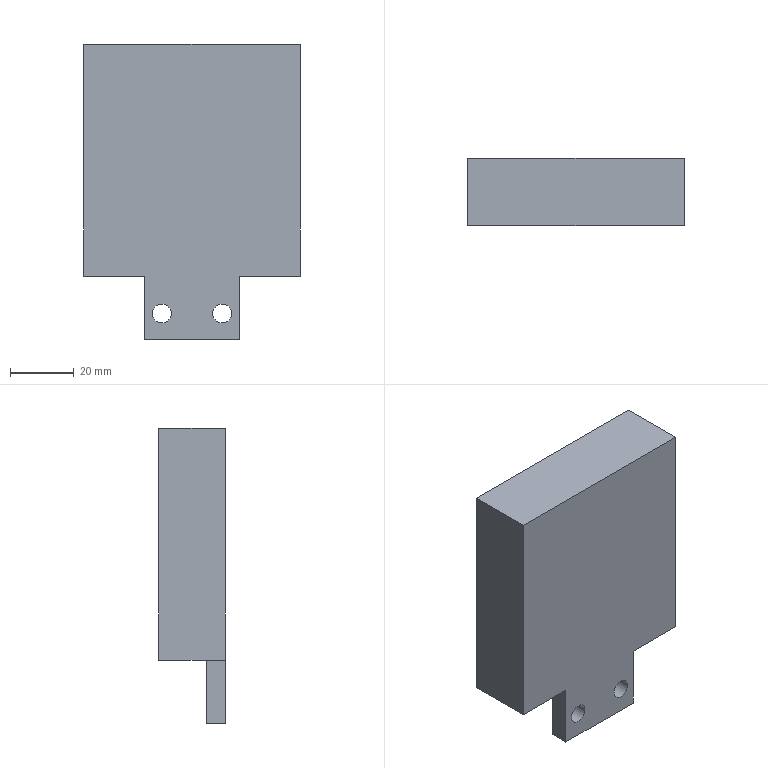Part | SolidWorks | features ICE 2, Extrusion 1 | 1 solid | 14 faces | box 68 x 21 x 93 mm | volume 107516 mm3 | plane 10 | cylinder 4 | commonest cylinder face diameters 6 x4
STEP:
#1=CARTESIAN_POINT('',(6.5,0.,-48.257));
#2=VERTEX_POINT('',#1);
#3=CARTESIAN_POINT('',(12.5,0.,-48.257));
#4=VERTEX_POINT('',#3);
#5=CARTESIAN_POINT('',(9.5,0.,-48.257));
#6=DIRECTION('',(0.,-1.,0.));
#7=DIRECTION('',(0.,0.,-1.));
#8=AXIS2_PLACEMENT_3D('',#5,#6,#7);
#9=CIRCLE('',#8,3.);
#10=EDGE_CURVE('',#2,#4,#9,.T.);
#11=ORIENTED_EDGE('',*,*,#10,.T.);
#12=CARTESIAN_POINT('',(12.5,6.02,-48.257));
#13=VERTEX_POINT('',#12);
#14=CARTESIAN_POINT('',(12.5,-13.98,-48.257));
#15=DIRECTION('',(0.,1.,0.));
#16=VECTOR('',#15,1000.);
#17=LINE('',#14,#16);
#18=EDGE_CURVE('',#4,#13,#17,.T.);
#19=ORIENTED_EDGE('',*,*,#18,.T.);
#20=CARTESIAN_POINT('',(6.5,6.02,-48.257));
#21=VERTEX_POINT('',#20);
#22=CARTESIAN_POINT('',(9.5,6.02,-48.257));
#23=DIRECTION('',(0.,1.,0.));
#24=DIRECTION('',(-1.,0.,0.));
#25=AXIS2_PLACEMENT_3D('',#22,#23,#24);
#26=CIRCLE('',#25,3.);
#27=EDGE_CURVE('',#13,#21,#26,.T.);
#28=ORIENTED_EDGE('',*,*,#27,.T.);
#29=CARTESIAN_POINT('',(6.5,-13.98,-48.257));
#30=DIRECTION('',(0.,1.,0.));
#31=VECTOR('',#30,1000.);
#32=LINE('',#29,#31);
#33=EDGE_CURVE('',#2,#21,#32,.T.);
#34=ORIENTED_EDGE('',*,*,#33,.F.);
#35=EDGE_LOOP('',(#11,#19,#28,#34));
#36=FACE_OUTER_BOUND('',#35,.T.);
#37=CARTESIAN_POINT('',(9.5,-13.98,-48.257));
#38=DIRECTION('',(0.,1.,0.));
#39=DIRECTION('',(-1.,0.,0.));
#40=AXIS2_PLACEMENT_3D('',#37,#38,#39);
#41=CYLINDRICAL_SURFACE('',#40,3.);
#42=ADVANCED_FACE('',(#36),#41,.F.);
#43=CARTESIAN_POINT('',(-12.5,0.,-48.257));
#44=VERTEX_POINT('',#43);
#45=CARTESIAN_POINT('',(-6.5,0.,-48.257));
#46=VERTEX_POINT('',#45);
#47=CARTESIAN_POINT('',(-9.5,0.,-48.257));
#48=DIRECTION('',(0.,-1.,0.));
#49=DIRECTION('',(0.,0.,-1.));
#50=AXIS2_PLACEMENT_3D('',#47,#48,#49);
#51=CIRCLE('',#50,3.);
#52=EDGE_CURVE('',#44,#46,#51,.T.);
#53=ORIENTED_EDGE('',*,*,#52,.T.);
#54=CARTESIAN_POINT('',(-6.5,6.02,-48.257));
#55=VERTEX_POINT('',#54);
#56=CARTESIAN_POINT('',(-6.5,-13.98,-48.257));
#57=DIRECTION('',(0.,1.,0.));
#58=VECTOR('',#57,1000.);
#59=LINE('',#56,#58);
#60=EDGE_CURVE('',#46,#55,#59,.T.);
#61=ORIENTED_EDGE('',*,*,#60,.T.);
#62=CARTESIAN_POINT('',(-12.5,6.02,-48.257));
#63=VERTEX_POINT('',#62);
#64=CARTESIAN_POINT('',(-9.5,6.02,-48.257));
#65=DIRECTION('',(0.,1.,0.));
#66=DIRECTION('',(-1.,0.,0.));
#67=AXIS2_PLACEMENT_3D('',#64,#65,#66);
#68=CIRCLE('',#67,3.);
#69=EDGE_CURVE('',#55,#63,#68,.T.);
#70=ORIENTED_EDGE('',*,*,#69,.T.);
#71=CARTESIAN_POINT('',(-12.5,-13.98,-48.257));
#72=DIRECTION('',(0.,1.,0.));
#73=VECTOR('',#72,1000.);
#74=LINE('',#71,#73);
#75=EDGE_CURVE('',#44,#63,#74,.T.);
#76=ORIENTED_EDGE('',*,*,#75,.F.);
#77=EDGE_LOOP('',(#53,#61,#70,#76));
#78=FACE_OUTER_BOUND('',#77,.T.);
#79=CARTESIAN_POINT('',(-9.5,-13.98,-48.257));
#80=DIRECTION('',(0.,1.,0.));
#81=DIRECTION('',(-1.,0.,0.));
#82=AXIS2_PLACEMENT_3D('',#79,#80,#81);
#83=CYLINDRICAL_SURFACE('',#82,3.);
#84=ADVANCED_FACE('',(#78),#83,.F.);
#85=CARTESIAN_POINT('',(-15.,0.,-36.5));
#86=VERTEX_POINT('',#85);
#87=CARTESIAN_POINT('',(-15.,6.02,-36.5));
#88=VERTEX_POINT('',#87);
#89=CARTESIAN_POINT('',(-15.,0.,-36.5));
#90=DIRECTION('',(0.,1.,0.));
#91=VECTOR('',#90,1000.);
#92=LINE('',#89,#91);
#93=EDGE_CURVE('',#86,#88,#92,.T.);
#94=ORIENTED_EDGE('',*,*,#93,.F.);
#95=CARTESIAN_POINT('',(-34.,0.,-36.5));
#96=VERTEX_POINT('',#95);
#97=CARTESIAN_POINT('',(-34.,0.,-36.5));
#98=DIRECTION('',(-1.,0.,0.));
#99=VECTOR('',#98,1000.);
#100=LINE('',#97,#99);
#101=EDGE_CURVE('',#86,#96,#100,.T.);
#102=ORIENTED_EDGE('',*,*,#101,.T.);
#103=CARTESIAN_POINT('',(-34.,21.,-36.5));
#104=VERTEX_POINT('',#103);
#105=CARTESIAN_POINT('',(-34.,21.,-36.5));
#106=DIRECTION('',(0.,-1.,0.));
#107=VECTOR('',#106,1000.);
#108=LINE('',#105,#107);
#109=EDGE_CURVE('',#104,#96,#108,.T.);
#110=ORIENTED_EDGE('',*,*,#109,.F.);
#111=CARTESIAN_POINT('',(34.,21.,-36.5));
#112=VERTEX_POINT('',#111);
#113=CARTESIAN_POINT('',(-34.,21.,-36.5));
#114=DIRECTION('',(-1.,0.,0.));
#115=VECTOR('',#114,1000.);
#116=LINE('',#113,#115);
#117=EDGE_CURVE('',#112,#104,#116,.T.);
#118=ORIENTED_EDGE('',*,*,#117,.F.);
#119=CARTESIAN_POINT('',(34.,0.,-36.5));
#120=VERTEX_POINT('',#119);
#121=CARTESIAN_POINT('',(34.,21.,-36.5));
#122=DIRECTION('',(0.,-1.,0.));
#123=VECTOR('',#122,1000.);
#124=LINE('',#121,#123);
#125=EDGE_CURVE('',#112,#120,#124,.T.);
#126=ORIENTED_EDGE('',*,*,#125,.T.);
#127=CARTESIAN_POINT('',(15.,0.,-36.5));
#128=VERTEX_POINT('',#127);
#129=CARTESIAN_POINT('',(-34.,0.,-36.5));
#130=DIRECTION('',(-1.,0.,0.));
#131=VECTOR('',#130,1000.);
#132=LINE('',#129,#131);
#133=EDGE_CURVE('',#120,#128,#132,.T.);
#134=ORIENTED_EDGE('',*,*,#133,.T.);
#135=CARTESIAN_POINT('',(15.,6.02,-36.5));
#136=VERTEX_POINT('',#135);
#137=CARTESIAN_POINT('',(15.,0.,-36.5));
#138=DIRECTION('',(0.,-1.,0.));
#139=VECTOR('',#138,1000.);
#140=LINE('',#137,#139);
#141=EDGE_CURVE('',#136,#128,#140,.T.);
#142=ORIENTED_EDGE('',*,*,#141,.F.);
#143=CARTESIAN_POINT('',(15.,6.02,-36.5));
#144=DIRECTION('',(1.,0.,0.));
#145=VECTOR('',#144,1000.);
#146=LINE('',#143,#145);
#147=EDGE_CURVE('',#88,#136,#146,.T.);
#148=ORIENTED_EDGE('',*,*,#147,.F.);
#149=EDGE_LOOP('',(#94,#102,#110,#118,#126,#134,#142,#148));
#150=FACE_OUTER_BOUND('',#149,.T.);
#151=CARTESIAN_POINT('',(-34.,21.,-36.5));
#152=DIRECTION('',(0.,0.,1.));
#153=DIRECTION('',(1.,0.,0.));
#154=AXIS2_PLACEMENT_3D('',#151,#152,#153);
#155=PLANE('',#154);
#156=ADVANCED_FACE('',(#150),#155,.F.);
#157=CARTESIAN_POINT('',(34.,0.,36.5));
#158=VERTEX_POINT('',#157);
#159=CARTESIAN_POINT('',(34.,0.,36.5));
#160=DIRECTION('',(0.,0.,-1.));
#161=VECTOR('',#160,1000.);
#162=LINE('',#159,#161);
#163=EDGE_CURVE('',#158,#120,#162,.T.);
#164=ORIENTED_EDGE('',*,*,#163,.T.);
#165=ORIENTED_EDGE('',*,*,#125,.F.);
#166=CARTESIAN_POINT('',(34.,21.,36.5));
#167=VERTEX_POINT('',#166);
#168=CARTESIAN_POINT('',(34.,21.,36.5));
#169=DIRECTION('',(0.,0.,-1.));
#170=VECTOR('',#169,1000.);
#171=LINE('',#168,#170);
#172=EDGE_CURVE('',#167,#112,#171,.T.);
#173=ORIENTED_EDGE('',*,*,#172,.F.);
#174=CARTESIAN_POINT('',(34.,21.,36.5));
#175=DIRECTION('',(0.,-1.,0.));
#176=VECTOR('',#175,1000.);
#177=LINE('',#174,#176);
#178=EDGE_CURVE('',#167,#158,#177,.T.);
#179=ORIENTED_EDGE('',*,*,#178,.T.);
#180=EDGE_LOOP('',(#164,#165,#173,#179));
#181=FACE_OUTER_BOUND('',#180,.T.);
#182=CARTESIAN_POINT('',(34.,21.,36.5));
#183=DIRECTION('',(-1.,0.,0.));
#184=DIRECTION('',(0.,0.,1.));
#185=AXIS2_PLACEMENT_3D('',#182,#183,#184);
#186=PLANE('',#185);
#187=ADVANCED_FACE('',(#181),#186,.F.);
#188=CARTESIAN_POINT('',(-34.,0.,36.5));
#189=VERTEX_POINT('',#188);
#190=CARTESIAN_POINT('',(-34.,0.,36.5));
#191=DIRECTION('',(0.,0.,1.));
#192=VECTOR('',#191,1000.);
#193=LINE('',#190,#192);
#194=EDGE_CURVE('',#96,#189,#193,.T.);
#195=ORIENTED_EDGE('',*,*,#194,.T.);
#196=CARTESIAN_POINT('',(-34.,21.,36.5));
#197=VERTEX_POINT('',#196);
#198=CARTESIAN_POINT('',(-34.,21.,36.5));
#199=DIRECTION('',(0.,-1.,0.));
#200=VECTOR('',#199,1000.);
#201=LINE('',#198,#200);
#202=EDGE_CURVE('',#197,#189,#201,.T.);
#203=ORIENTED_EDGE('',*,*,#202,.F.);
#204=CARTESIAN_POINT('',(-34.,21.,36.5));
#205=DIRECTION('',(0.,0.,1.));
#206=VECTOR('',#205,1000.);
#207=LINE('',#204,#206);
#208=EDGE_CURVE('',#104,#197,#207,.T.);
#209=ORIENTED_EDGE('',*,*,#208,.F.);
#210=ORIENTED_EDGE('',*,*,#109,.T.);
#211=EDGE_LOOP('',(#195,#203,#209,#210));
#212=FACE_OUTER_BOUND('',#211,.T.);
#213=CARTESIAN_POINT('',(-34.,21.,36.5));
#214=DIRECTION('',(1.,0.,0.));
#215=DIRECTION('',(0.,0.,-1.));
#216=AXIS2_PLACEMENT_3D('',#213,#214,#215);
#217=PLANE('',#216);
#218=ADVANCED_FACE('',(#212),#217,.F.);
#219=CARTESIAN_POINT('',(-34.,0.,36.5));
#220=DIRECTION('',(1.,0.,0.));
#221=VECTOR('',#220,1000.);
#222=LINE('',#219,#221);
#223=EDGE_CURVE('',#189,#158,#222,.T.);
#224=ORIENTED_EDGE('',*,*,#223,.T.);
#225=ORIENTED_EDGE('',*,*,#178,.F.);
#226=CARTESIAN_POINT('',(-34.,21.,36.5));
#227=DIRECTION('',(1.,0.,0.));
#228=VECTOR('',#227,1000.);
#229=LINE('',#226,#228);
#230=EDGE_CURVE('',#197,#167,#229,.T.);
#231=ORIENTED_EDGE('',*,*,#230,.F.);
#232=ORIENTED_EDGE('',*,*,#202,.T.);
#233=EDGE_LOOP('',(#224,#225,#231,#232));
#234=FACE_OUTER_BOUND('',#233,.T.);
#235=CARTESIAN_POINT('',(-34.,21.,36.5));
#236=DIRECTION('',(0.,0.,-1.));
#237=DIRECTION('',(-1.,0.,0.));
#238=AXIS2_PLACEMENT_3D('',#235,#236,#237);
#239=PLANE('',#238);
#240=ADVANCED_FACE('',(#234),#239,.F.);
#241=ORIENTED_EDGE('',*,*,#172,.T.);
#242=ORIENTED_EDGE('',*,*,#117,.T.);
#243=ORIENTED_EDGE('',*,*,#208,.T.);
#244=ORIENTED_EDGE('',*,*,#230,.T.);
#245=EDGE_LOOP('',(#241,#242,#243,#244));
#246=FACE_OUTER_BOUND('',#245,.T.);
#247=CARTESIAN_POINT('',(0.,21.,0.));
#248=DIRECTION('',(0.,-1.,0.));
#249=DIRECTION('',(0.,0.,-1.));
#250=AXIS2_PLACEMENT_3D('',#247,#248,#249);
#251=PLANE('',#250);
#252=ADVANCED_FACE('',(#246),#251,.F.);
#253=ORIENTED_EDGE('',*,*,#10,.F.);
#254=CARTESIAN_POINT('',(9.5,0.,-48.257));
#255=DIRECTION('',(0.,-1.,0.));
#256=DIRECTION('',(0.,0.,-1.));
#257=AXIS2_PLACEMENT_3D('',#254,#255,#256);
#258=CIRCLE('',#257,3.);
#259=EDGE_CURVE('',#4,#2,#258,.T.);
#260=ORIENTED_EDGE('',*,*,#259,.F.);
#261=EDGE_LOOP('',(#253,#260));
#262=FACE_BOUND('',#261,.T.);
#263=ORIENTED_EDGE('',*,*,#52,.F.);
#264=CARTESIAN_POINT('',(-9.5,0.,-48.257));
#265=DIRECTION('',(0.,-1.,0.));
#266=DIRECTION('',(0.,0.,-1.));
#267=AXIS2_PLACEMENT_3D('',#264,#265,#266);
#268=CIRCLE('',#267,3.);
#269=EDGE_CURVE('',#46,#44,#268,.T.);
#270=ORIENTED_EDGE('',*,*,#269,.F.);
#271=EDGE_LOOP('',(#263,#270));
#272=FACE_BOUND('',#271,.T.);
#273=ORIENTED_EDGE('',*,*,#163,.F.);
#274=ORIENTED_EDGE('',*,*,#223,.F.);
#275=ORIENTED_EDGE('',*,*,#194,.F.);
#276=ORIENTED_EDGE('',*,*,#101,.F.);
#277=CARTESIAN_POINT('',(-15.,0.,-56.5));
#278=VERTEX_POINT('',#277);
#279=CARTESIAN_POINT('',(-15.,0.,-56.5));
#280=DIRECTION('',(0.,0.,1.));
#281=VECTOR('',#280,1000.);
#282=LINE('',#279,#281);
#283=EDGE_CURVE('',#278,#86,#282,.T.);
#284=ORIENTED_EDGE('',*,*,#283,.F.);
#285=CARTESIAN_POINT('',(15.,0.,-56.5));
#286=VERTEX_POINT('',#285);
#287=CARTESIAN_POINT('',(15.,0.,-56.5));
#288=DIRECTION('',(-1.,0.,0.));
#289=VECTOR('',#288,1000.);
#290=LINE('',#287,#289);
#291=EDGE_CURVE('',#286,#278,#290,.T.);
#292=ORIENTED_EDGE('',*,*,#291,.F.);
#293=CARTESIAN_POINT('',(15.,0.,-56.5));
#294=DIRECTION('',(0.,0.,1.));
#295=VECTOR('',#294,1000.);
#296=LINE('',#293,#295);
#297=EDGE_CURVE('',#286,#128,#296,.T.);
#298=ORIENTED_EDGE('',*,*,#297,.T.);
#299=ORIENTED_EDGE('',*,*,#133,.F.);
#300=EDGE_LOOP('',(#273,#274,#275,#276,#284,#292,#298,#299));
#301=FACE_OUTER_BOUND('',#300,.T.);
#302=CARTESIAN_POINT('',(0.,0.,0.));
#303=DIRECTION('',(0.,-1.,0.));
#304=DIRECTION('',(0.,0.,-1.));
#305=AXIS2_PLACEMENT_3D('',#302,#303,#304);
#306=PLANE('',#305);
#307=ADVANCED_FACE('',(#262,#272,#301),#306,.T.);
#308=ORIENTED_EDGE('',*,*,#93,.T.);
#309=CARTESIAN_POINT('',(-15.,6.02,-56.5));
#310=VERTEX_POINT('',#309);
#311=CARTESIAN_POINT('',(-15.,6.02,-56.5));
#312=DIRECTION('',(0.,0.,1.));
#313=VECTOR('',#312,1000.);
#314=LINE('',#311,#313);
#315=EDGE_CURVE('',#310,#88,#314,.T.);
#316=ORIENTED_EDGE('',*,*,#315,.F.);
#317=CARTESIAN_POINT('',(-15.,0.,-56.5));
#318=DIRECTION('',(0.,1.,0.));
#319=VECTOR('',#318,1000.);
#320=LINE('',#317,#319);
#321=EDGE_CURVE('',#278,#310,#320,.T.);
#322=ORIENTED_EDGE('',*,*,#321,.F.);
#323=ORIENTED_EDGE('',*,*,#283,.T.);
#324=EDGE_LOOP('',(#308,#316,#322,#323));
#325=FACE_OUTER_BOUND('',#324,.T.);
#326=CARTESIAN_POINT('',(-15.,0.,-56.5));
#327=DIRECTION('',(1.,0.,0.));
#328=DIRECTION('',(0.,0.,-1.));
#329=AXIS2_PLACEMENT_3D('',#326,#327,#328);
#330=PLANE('',#329);
#331=ADVANCED_FACE('',(#325),#330,.F.);
#332=CARTESIAN_POINT('',(9.5,6.02,-48.257));
#333=DIRECTION('',(0.,1.,0.));
#334=DIRECTION('',(-1.,0.,0.));
#335=AXIS2_PLACEMENT_3D('',#332,#333,#334);
#336=CIRCLE('',#335,3.);
#337=EDGE_CURVE('',#21,#13,#336,.T.);
#338=ORIENTED_EDGE('',*,*,#337,.F.);
#339=ORIENTED_EDGE('',*,*,#27,.F.);
#340=EDGE_LOOP('',(#338,#339));
#341=FACE_BOUND('',#340,.T.);
#342=CARTESIAN_POINT('',(-9.5,6.02,-48.257));
#343=DIRECTION('',(0.,1.,0.));
#344=DIRECTION('',(-1.,0.,0.));
#345=AXIS2_PLACEMENT_3D('',#342,#343,#344);
#346=CIRCLE('',#345,3.);
#347=EDGE_CURVE('',#63,#55,#346,.T.);
#348=ORIENTED_EDGE('',*,*,#347,.F.);
#349=ORIENTED_EDGE('',*,*,#69,.F.);
#350=EDGE_LOOP('',(#348,#349));
#351=FACE_BOUND('',#350,.T.);
#352=ORIENTED_EDGE('',*,*,#147,.T.);
#353=CARTESIAN_POINT('',(15.,6.02,-56.5));
#354=VERTEX_POINT('',#353);
#355=CARTESIAN_POINT('',(15.,6.02,-56.5));
#356=DIRECTION('',(0.,0.,1.));
#357=VECTOR('',#356,1000.);
#358=LINE('',#355,#357);
#359=EDGE_CURVE('',#354,#136,#358,.T.);
#360=ORIENTED_EDGE('',*,*,#359,.F.);
#361=CARTESIAN_POINT('',(15.,6.02,-56.5));
#362=DIRECTION('',(1.,0.,0.));
#363=VECTOR('',#362,1000.);
#364=LINE('',#361,#363);
#365=EDGE_CURVE('',#310,#354,#364,.T.);
#366=ORIENTED_EDGE('',*,*,#365,.F.);
#367=ORIENTED_EDGE('',*,*,#315,.T.);
#368=EDGE_LOOP('',(#352,#360,#366,#367));
#369=FACE_OUTER_BOUND('',#368,.T.);
#370=CARTESIAN_POINT('',(15.,6.02,-56.5));
#371=DIRECTION('',(0.,-1.,0.));
#372=DIRECTION('',(1.,0.,0.));
#373=AXIS2_PLACEMENT_3D('',#370,#371,#372);
#374=PLANE('',#373);
#375=ADVANCED_FACE('',(#341,#351,#369),#374,.F.);
#376=ORIENTED_EDGE('',*,*,#141,.T.);
#377=ORIENTED_EDGE('',*,*,#297,.F.);
#378=CARTESIAN_POINT('',(15.,0.,-56.5));
#379=DIRECTION('',(0.,-1.,0.));
#380=VECTOR('',#379,1000.);
#381=LINE('',#378,#380);
#382=EDGE_CURVE('',#354,#286,#381,.T.);
#383=ORIENTED_EDGE('',*,*,#382,.F.);
#384=ORIENTED_EDGE('',*,*,#359,.T.);
#385=EDGE_LOOP('',(#376,#377,#383,#384));
#386=FACE_OUTER_BOUND('',#385,.T.);
#387=CARTESIAN_POINT('',(15.,0.,-56.5));
#388=DIRECTION('',(-1.,0.,0.));
#389=DIRECTION('',(0.,0.,1.));
#390=AXIS2_PLACEMENT_3D('',#387,#388,#389);
#391=PLANE('',#390);
#392=ADVANCED_FACE('',(#386),#391,.F.);
#393=ORIENTED_EDGE('',*,*,#321,.T.);
#394=ORIENTED_EDGE('',*,*,#365,.T.);
#395=ORIENTED_EDGE('',*,*,#382,.T.);
#396=ORIENTED_EDGE('',*,*,#291,.T.);
#397=EDGE_LOOP('',(#393,#394,#395,#396));
#398=FACE_OUTER_BOUND('',#397,.T.);
#399=CARTESIAN_POINT('',(0.,0.,-56.5));
#400=DIRECTION('',(0.,0.,1.));
#401=DIRECTION('',(1.,0.,0.));
#402=AXIS2_PLACEMENT_3D('',#399,#400,#401);
#403=PLANE('',#402);
#404=ADVANCED_FACE('',(#398),#403,.F.);
#405=ORIENTED_EDGE('',*,*,#60,.F.);
#406=ORIENTED_EDGE('',*,*,#269,.T.);
#407=ORIENTED_EDGE('',*,*,#75,.T.);
#408=ORIENTED_EDGE('',*,*,#347,.T.);
#409=EDGE_LOOP('',(#405,#406,#407,#408));
#410=FACE_OUTER_BOUND('',#409,.T.);
#411=CARTESIAN_POINT('',(-9.5,-13.98,-48.257));
#412=DIRECTION('',(0.,1.,0.));
#413=DIRECTION('',(-1.,0.,0.));
#414=AXIS2_PLACEMENT_3D('',#411,#412,#413);
#415=CYLINDRICAL_SURFACE('',#414,3.);
#416=ADVANCED_FACE('',(#410),#415,.F.);
#417=ORIENTED_EDGE('',*,*,#18,.F.);
#418=ORIENTED_EDGE('',*,*,#259,.T.);
#419=ORIENTED_EDGE('',*,*,#33,.T.);
#420=ORIENTED_EDGE('',*,*,#337,.T.);
#421=EDGE_LOOP('',(#417,#418,#419,#420));
#422=FACE_OUTER_BOUND('',#421,.T.);
#423=CARTESIAN_POINT('',(9.5,-13.98,-48.257));
#424=DIRECTION('',(0.,1.,0.));
#425=DIRECTION('',(-1.,0.,0.));
#426=AXIS2_PLACEMENT_3D('',#423,#424,#425);
#427=CYLINDRICAL_SURFACE('',#426,3.);
#428=ADVANCED_FACE('',(#422),#427,.F.);
#429=CLOSED_SHELL('',(#42,#84,#156,#187,#218,#240,#252,#307,#331,#375,#392,#404,#416,#428));
#430=MANIFOLD_SOLID_BREP('',#429);
#431=CARTESIAN_POINT('',(0.,0.,0.));
#432=DIRECTION('',(0.,0.,1.));
#433=DIRECTION('',(1.,0.,0.));
#434=AXIS2_PLACEMENT_3D('',#431,#432,#433);
#435=(LENGTH_UNIT()NAMED_UNIT(*)SI_UNIT(.MILLI.,.METRE.));
#436=UNCERTAINTY_MEASURE_WITH_UNIT(LENGTH_MEASURE(0.00001),#435,'','');
#437=(NAMED_UNIT(*)PLANE_ANGLE_UNIT()SI_UNIT($,.RADIAN.));
#438=(NAMED_UNIT(*)SI_UNIT($,.STERADIAN.)SOLID_ANGLE_UNIT());
#439=(GEOMETRIC_REPRESENTATION_CONTEXT(3)GLOBAL_UNCERTAINTY_ASSIGNED_CONTEXT((#436))GLOBAL_UNIT_ASSIGNED_CONTEXT((#435,#437,#438))REPRESENTATION_CONTEXT('',''));
#440=ADVANCED_BREP_SHAPE_REPRESENTATION('',(#430,#434),#439);